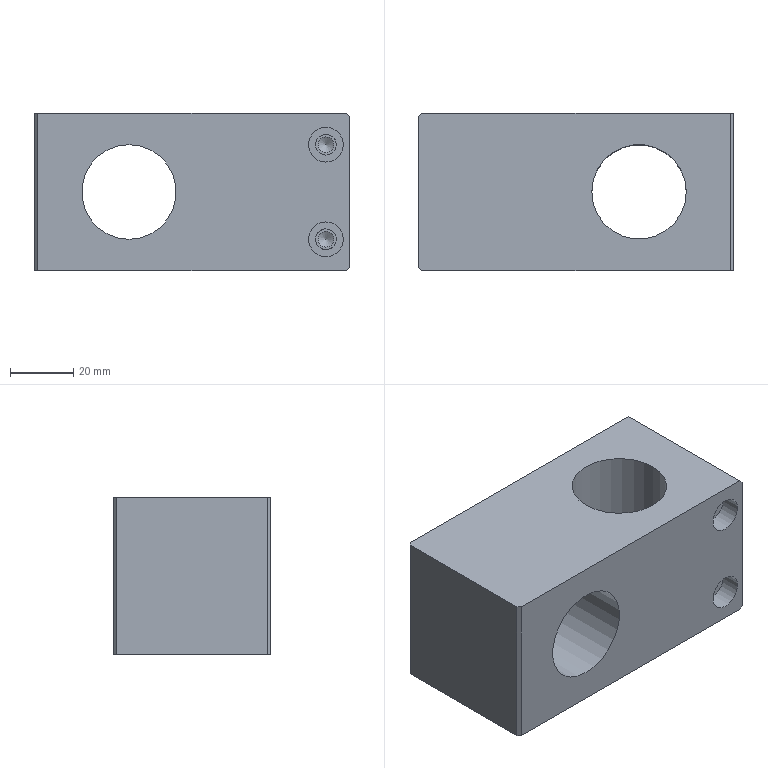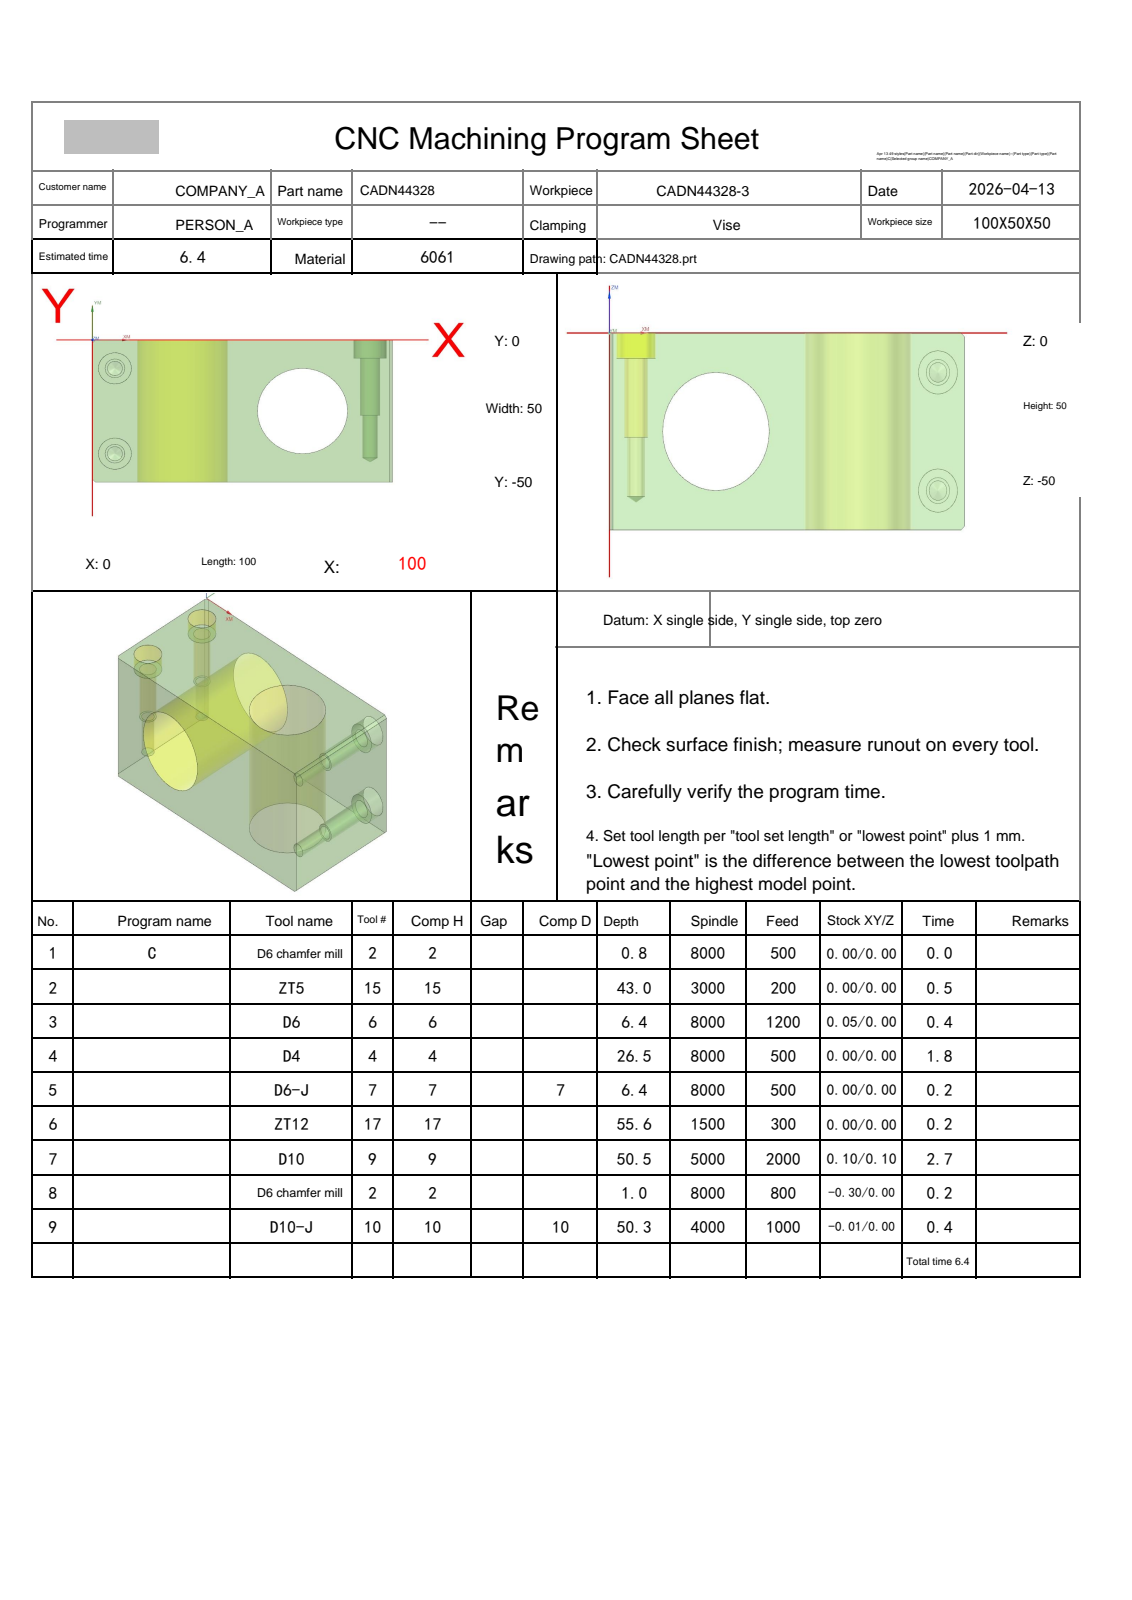NC program | NX | posted by the shop | part box 100 x 50 x 50 mm
Whole program:
%
O0001
(Machine time: 8.18 MIN)
(===Total Tool:8===)
(T2=D6 chamfer mill D=6. R=0. D- H02 Z=-1.   )
(T15=ZT5 D=5. DR_a=118 D- H15 Z=-43.  )
(T6=D6 D=6. R=0. D- H06 Z=-6.4  )
(T4=D4 D=4. R=0. D- H04 Z=-26.5 )
(T7=D6-J D=6. R=0. D7 H07 Z=-6.4  )
(T17=ZT12 D=12. DR_a=118 D- H17 Z=-55.61)
(T9=D10 D=10. R=0. D- H09 Z=-50.5 )
(T10=D10-J D=10. R=0. D10 H10 Z=-50.3 )
G80 G90 G17 G49 G40
G91 G28 Z0
M01
N1 T02 M06
(D6 chamfer mill D=6. R=0. H=02 ce=0.00 di=0.00)
G00 G90 G54 X7.5 Y-40. M03 S8000
G43 H02 Z20.
M08
G98 G81 X7.5 Y-40. Z-.8 R1. F500.
Y-10.
G80
G00 Z20.
G00 G90 X70. Y-25. M03 S8000
Z20.
G98 G82 X70. Y-25. Z-.8 R1. F500.
G80
G00 Z20.
G91 G28 Z0.0
M05
M09
G91 G28 Z0.0
M01
N2 T15 M06
(ZT5 D=5. DR_a=118 H=15)
G00 G90 G54 X7.5 Y-40. M03 S3000
G43 H15 Z20.
M08
G98 G83 X7.5 Y-40. Z-43.002 R1. F200. Q2.
Y-10.
G80
G00 Z20.
G91 G28 Z0.0
M05
M09
G91 G28 Z0.0
M01
N3 T06 M06
(D6 D=6. R=0. H=06 ce=0.05 di=0.00)
G00 G90 G54 X7.5 Y-40. M03 S8000
G43 H06 Z20.
M08
Z.5
G03 X8.725 Y-41.225 I1.225 J0.0 F1200.
X9.95 Y-40. I0.0 J1.225
X9.95 Y-40. Z0.0 I-2.45 J0.0
X9.95 Y-40. Z-.5 I-2.45 J0.0
X9.95 Y-40. Z-1. I-2.45 J0.0
X9.95 Y-40. Z-1.5 I-2.45 J0.0
X9.95 Y-40. Z-2. I-2.45 J0.0
X9.95 Y-40. Z-2.5 I-2.45 J0.0
X9.95 Y-40. Z-3. I-2.45 J0.0
X9.95 Y-40. Z-3.5 I-2.45 J0.0
X9.95 Y-40. Z-4. I-2.45 J0.0
X9.95 Y-40. Z-4.5 I-2.45 J0.0
X9.95 Y-40. Z-5. I-2.45 J0.0
X9.95 Y-40. Z-5.5 I-2.45 J0.0
X9.95 Y-40. Z-6. I-2.45 J0.0
X8.257 Y-42.33 Z-6.4 I-2.45 J0.0
X9.95 Y-40. I-.757 J2.33
X7.5 Y-37.55 I-2.45 J0.0
X5.05 Y-40. I0.0 J-2.45
X7.5 Y-42.45 I2.45 J0.0
X8.257 Y-42.33 I0.0 J2.45
X9.104 Y-41.165 I-.379 J1.165
X7.879 Y-39.94 I-1.225 J0.0
X7.5 Y-40. I0.0 J-1.225
G00 Z20.
Y-10.
Z.5
G03 X8.725 Y-11.225 I1.225 J0.0
X9.95 Y-10. I0.0 J1.225
X9.95 Y-10. Z0.0 I-2.45 J0.0
X9.95 Y-10. Z-.5 I-2.45 J0.0
X9.95 Y-10. Z-1. I-2.45 J0.0
X9.95 Y-10. Z-1.5 I-2.45 J0.0
X9.95 Y-10. Z-2. I-2.45 J0.0
X9.95 Y-10. Z-2.5 I-2.45 J0.0
X9.95 Y-10. Z-3. I-2.45 J0.0
X9.95 Y-10. Z-3.5 I-2.45 J0.0
X9.95 Y-10. Z-4. I-2.45 J0.0
X9.95 Y-10. Z-4.5 I-2.45 J0.0
X9.95 Y-10. Z-5. I-2.45 J0.0
X9.95 Y-10. Z-5.5 I-2.45 J0.0
X9.95 Y-10. Z-6. I-2.45 J0.0
X8.257 Y-12.33 Z-6.4 I-2.45 J0.0
X9.95 Y-10. I-.757 J2.33
X7.5 Y-7.55 I-2.45 J0.0
X5.05 Y-10. I0.0 J-2.45
X7.5 Y-12.45 I2.45 J0.0
X8.257 Y-12.33 I0.0 J2.45
X9.104 Y-11.165 I-.379 J1.165
X7.879 Y-9.94 I-1.225 J0.0
X7.5 Y-10. I0.0 J-1.225
G00 Z20.
G91 G28 Z0.0
M05
M09
G91 G28 Z0.0
M01
N4 T04 M06
(D4 D=4. R=0. H=04 ce=0.00 di=0.00)
G00 G90 G54 X7.5 Y-40. M03 S8000
G43 H04 Z20.
M08
Z-5.9
G03 X8.15 Y-40.65 I.65 J0.0 F500.
X8.8 Y-40. I0.0 J.65
X8.8 Y-40. Z-6.3 I-1.3 J0.0
X8.8 Y-40. Z-6.7 I-1.3 J0.0
X8.8 Y-40. Z-7.1 I-1.3 J0.0
X8.8 Y-40. Z-7.5 I-1.3 J0.0
X8.8 Y-40. Z-7.9 I-1.3 J0.0
X8.8 Y-40. Z-8.3 I-1.3 J0.0
X8.8 Y-40. Z-8.7 I-1.3 J0.0
X8.8 Y-40. Z-9.1 I-1.3 J0.0
X8.8 Y-40. Z-9.5 I-1.3 J0.0
X8.8 Y-40. Z-9.9 I-1.3 J0.0
X8.8 Y-40. Z-10.3 I-1.3 J0.0
X8.8 Y-40. Z-10.7 I-1.3 J0.0
X8.8 Y-40. Z-11.1 I-1.3 J0.0
X8.8 Y-40. Z-11.5 I-1.3 J0.0
X8.8 Y-40. Z-11.9 I-1.3 J0.0
X8.8 Y-40. Z-12.3 I-1.3 J0.0
X8.8 Y-40. Z-12.7 I-1.3 J0.0
X8.8 Y-40. Z-13.1 I-1.3 J0.0
X8.8 Y-40. Z-13.5 I-1.3 J0.0
X8.8 Y-40. Z-13.9 I-1.3 J0.0
X8.8 Y-40. Z-14.3 I-1.3 J0.0
X8.8 Y-40. Z-14.7 I-1.3 J0.0
X8.8 Y-40. Z-15.1 I-1.3 J0.0
X8.8 Y-40. Z-15.5 I-1.3 J0.0
X8.8 Y-40. Z-15.9 I-1.3 J0.0
X8.8 Y-40. Z-16.3 I-1.3 J0.0
X8.8 Y-40. Z-16.7 I-1.3 J0.0
X8.8 Y-40. Z-17.1 I-1.3 J0.0
X8.8 Y-40. Z-17.5 I-1.3 J0.0
X8.8 Y-40. Z-17.9 I-1.3 J0.0
X8.8 Y-40. Z-18.3 I-1.3 J0.0
X8.8 Y-40. Z-18.7 I-1.3 J0.0
X8.8 Y-40. Z-19.1 I-1.3 J0.0
X8.8 Y-40. Z-19.5 I-1.3 J0.0
X8.8 Y-40. Z-19.9 I-1.3 J0.0
X8.8 Y-40. Z-20.3 I-1.3 J0.0
X8.8 Y-40. Z-20.7 I-1.3 J0.0
X8.8 Y-40. Z-21.1 I-1.3 J0.0
X8.8 Y-40. Z-21.5 I-1.3 J0.0
X8.8 Y-40. Z-21.9 I-1.3 J0.0
X8.8 Y-40. Z-22.3 I-1.3 J0.0
X8.8 Y-40. Z-22.7 I-1.3 J0.0
X8.8 Y-40. Z-23.1 I-1.3 J0.0
X8.8 Y-40. Z-23.5 I-1.3 J0.0
X8.8 Y-40. Z-23.9 I-1.3 J0.0
X8.8 Y-40. Z-24.3 I-1.3 J0.0
X8.8 Y-40. Z-24.7 I-1.3 J0.0
X8.8 Y-40. Z-25.1 I-1.3 J0.0
X8.8 Y-40. Z-25.5 I-1.3 J0.0
X8.8 Y-40. Z-25.9 I-1.3 J0.0
X8.8 Y-40. Z-26.3 I-1.3 J0.0
X6.2 Y-40. Z-26.5 I-1.3 J0.0
X7.5 Y-41.3 I1.3 J0.0
X8.8 Y-40. I0.0 J1.3
X7.5 Y-38.7 I-1.3 J0.0
X6.2 Y-40. I0.0 J-1.3
X6.85 Y-40.65 I.65 J0.0
X7.5 Y-40. I0.0 J.65
G00 Z20.
Y-10.
Z-5.9
G03 X8.15 Y-10.65 I.65 J0.0
X8.8 Y-10. I0.0 J.65
X8.8 Y-10. Z-6.3 I-1.3 J0.0
X8.8 Y-10. Z-6.7 I-1.3 J0.0
X8.8 Y-10. Z-7.1 I-1.3 J0.0
X8.8 Y-10. Z-7.5 I-1.3 J0.0
X8.8 Y-10. Z-7.9 I-1.3 J0.0
X8.8 Y-10. Z-8.3 I-1.3 J0.0
X8.8 Y-10. Z-8.7 I-1.3 J0.0
X8.8 Y-10. Z-9.1 I-1.3 J0.0
X8.8 Y-10. Z-9.5 I-1.3 J0.0
X8.8 Y-10. Z-9.9 I-1.3 J0.0
X8.8 Y-10. Z-10.3 I-1.3 J0.0
X8.8 Y-10. Z-10.7 I-1.3 J0.0
X8.8 Y-10. Z-11.1 I-1.3 J0.0
X8.8 Y-10. Z-11.5 I-1.3 J0.0
X8.8 Y-10. Z-11.9 I-1.3 J0.0
X8.8 Y-10. Z-12.3 I-1.3 J0.0
X8.8 Y-10. Z-12.7 I-1.3 J0.0
X8.8 Y-10. Z-13.1 I-1.3 J0.0
X8.8 Y-10. Z-13.5 I-1.3 J0.0
X8.8 Y-10. Z-13.9 I-1.3 J0.0
X8.8 Y-10. Z-14.3 I-1.3 J0.0
X8.8 Y-10. Z-14.7 I-1.3 J0.0
X8.8 Y-10. Z-15.1 I-1.3 J0.0
X8.8 Y-10. Z-15.5 I-1.3 J0.0
X8.8 Y-10. Z-15.9 I-1.3 J0.0
X8.8 Y-10. Z-16.3 I-1.3 J0.0
X8.8 Y-10. Z-16.7 I-1.3 J0.0
X8.8 Y-10. Z-17.1 I-1.3 J0.0
X8.8 Y-10. Z-17.5 I-1.3 J0.0
X8.8 Y-10. Z-17.9 I-1.3 J0.0
X8.8 Y-10. Z-18.3 I-1.3 J0.0
X8.8 Y-10. Z-18.7 I-1.3 J0.0
X8.8 Y-10. Z-19.1 I-1.3 J0.0
X8.8 Y-10. Z-19.5 I-1.3 J0.0
X8.8 Y-10. Z-19.9 I-1.3 J0.0
X8.8 Y-10. Z-20.3 I-1.3 J0.0
X8.8 Y-10. Z-20.7 I-1.3 J0.0
X8.8 Y-10. Z-21.1 I-1.3 J0.0
X8.8 Y-10. Z-21.5 I-1.3 J0.0
X8.8 Y-10. Z-21.9 I-1.3 J0.0
X8.8 Y-10. Z-22.3 I-1.3 J0.0
X8.8 Y-10. Z-22.7 I-1.3 J0.0
X8.8 Y-10. Z-23.1 I-1.3 J0.0
X8.8 Y-10. Z-23.5 I-1.3 J0.0
X8.8 Y-10. Z-23.9 I-1.3 J0.0
X8.8 Y-10. Z-24.3 I-1.3 J0.0
X8.8 Y-10. Z-24.7 I-1.3 J0.0
X8.8 Y-10. Z-25.1 I-1.3 J0.0
X8.8 Y-10. Z-25.5 I-1.3 J0.0
X8.8 Y-10. Z-25.9 I-1.3 J0.0
X8.8 Y-10. Z-26.3 I-1.3 J0.0
X6.2 Y-10. Z-26.5 I-1.3 J0.0
X7.5 Y-11.3 I1.3 J0.0
X8.8 Y-10. I0.0 J1.3
X7.5 Y-8.7 I-1.3 J0.0
X6.2 Y-10. I0.0 J-1.3
X6.85 Y-10.65 I.65 J0.0
X7.5 Y-10. I0.0 J.65
G00 Z20.
G91 G28 Z0.0
M05
M09
G91 G28 Z0.0
M01
N5 T07 M06
(D6-J D=6. R=0. H=07 ce=0.00 di=0.00)
G00 G90 G54 X7.5 Y-40. M03 S8000
G43 H07 Z20.
M08
Z.5
G41 D07
G01 X7.532 Y-40.197 F500.
G03 X8.758 Y-41.242 I1.226 J.197
X10. Y-40. I0.0 J1.242
X10. Y-40. Z-4.5 I-2.5 J0.0
X5.678 Y-38.289 Z-6.4 I-2.5 J0.0
X5. Y-40. I1.822 J-1.711
X7.5 Y-42.5 I2.5 J0.0
X10. Y-40. I0.0 J2.5
X7.5 Y-37.5 I-2.5 J0.0
X5.678 Y-38.289 I0.0 J-2.5
X5.341 Y-39.139 I.905 J-.85
X6.583 Y-40.381 I1.242 J0.0
X7.342 Y-40.122 I0.0 J1.242
G01 G40 X7.5 Y-40.
G00 Z20.
Y-10.
Z.5
G41 D07
G01 X7.532 Y-10.197
G03 X8.758 Y-11.242 I1.226 J.197
X10. Y-10. I0.0 J1.242
X10. Y-10. Z-4.5 I-2.5 J0.0
X5.678 Y-8.289 Z-6.4 I-2.5 J0.0
X5. Y-10. I1.822 J-1.711
X7.5 Y-12.5 I2.5 J0.0
X10. Y-10. I0.0 J2.5
X7.5 Y-7.5 I-2.5 J0.0
X5.678 Y-8.289 I0.0 J-2.5
X5.341 Y-9.139 I.905 J-.85
X6.583 Y-10.381 I1.242 J0.0
X7.342 Y-10.122 I0.0 J1.242
G01 G40 X7.5 Y-10.
G00 Z20.
G91 G28 Z0.0
M05
M09
G91 G28 Z0.0
M01
N6 T17 M06
(ZT12 D=12. DR_a=118 H=17)
G00 G90 G54 X70. Y-25. M03 S1500
G43 H17 Z20.
M08
G98 G83 X70. Y-25. Z-55.605 R1. F300. Q3.
G80
G00 Z20.
G91 G28 Z0.0
M05
M09
G91 G28 Z0.0
M01
N7 T09 M06
(D10 D=10. R=0. H=09 ce=0.10 di=0.10)
G00 G90 G54 X60.729 Y-21.576 M03 S5000
G43 H09 Z20.
M08
Z1.
G01 X60.457 Y-22.256 Z.962 F2000.
X60.1 Y-24.229 Z.857
Y-25.771 Z.776
X60.457 Y-27.744 Z.671
X61.202 Y-29.604 Z.566
X62.306 Y-31.277 Z.461
X63.723 Y-32.694 Z.356
X65.396 Y-33.798 Z.251
X67.256 Y-34.543 Z.145
X69.229 Y-34.9 Z.04
X70. Z0.0
G03 X79.9 Y-25. Z-.149 I0.0 J9.9
X70. Y-15.1 Z-.297 I-9.9 J0.0
X60.1 Y-25. Z-.446 I0.0 J-9.9
X70. Y-34.9 Z-.594 I9.9 J0.0
X79.9 Y-25. Z-.743 I0.0 J9.9
X70. Y-15.1 Z-.891 I-9.9 J0.0
X60.1 Y-25. Z-1.04 I0.0 J-9.9
X70. Y-34.9 Z-1.188 I9.9 J0.0
X79.9 Y-25. Z-1.337 I0.0 J9.9
X70. Y-15.1 Z-1.485 I-9.9 J0.0
X60.1 Y-25. Z-1.634 I0.0 J-9.9
X70. Y-34.9 Z-1.782 I9.9 J0.0
X79.9 Y-25. Z-1.931 I0.0 J9.9
X70. Y-15.1 Z-2.079 I-9.9 J0.0
X60.1 Y-25. Z-2.228 I0.0 J-9.9
X70. Y-34.9 Z-2.376 I9.9 J0.0
X79.9 Y-25. Z-2.525 I0.0 J9.9
X70. Y-15.1 Z-2.674 I-9.9 J0.0
X60.1 Y-25. Z-2.822 I0.0 J-9.9
X70. Y-34.9 Z-2.971 I9.9 J0.0
X79.9 Y-25. Z-3.119 I0.0 J9.9
X70. Y-15.1 Z-3.268 I-9.9 J0.0
X60.1 Y-25. Z-3.416 I0.0 J-9.9
X70. Y-34.9 Z-3.565 I9.9 J0.0
X79.9 Y-25. Z-3.713 I0.0 J9.9
X70. Y-15.1 Z-3.862 I-9.9 J0.0
X60.1 Y-25. Z-4.01 I0.0 J-9.9
X70. Y-34.9 Z-4.159 I9.9 J0.0
X79.9 Y-25. Z-4.307 I0.0 J9.9
X70. Y-15.1 Z-4.456 I-9.9 J0.0
X60.1 Y-25. Z-4.604 I0.0 J-9.9
X70. Y-34.9 Z-4.753 I9.9 J0.0
X79.9 Y-25. Z-4.901 I0.0 J9.9
X70. Y-15.1 Z-5.05 I-9.9 J0.0
X60.1 Y-25. Z-5.199 I0.0 J-9.9
X70. Y-34.9 Z-5.347 I9.9 J0.0
X79.9 Y-25. Z-5.496 I0.0 J9.9
X70. Y-15.1 Z-5.644 I-9.9 J0.0
X60.1 Y-25. Z-5.793 I0.0 J-9.9
X70. Y-34.9 Z-5.941 I9.9 J0.0
X79.9 Y-25. Z-6.09 I0.0 J9.9
X70. Y-15.1 Z-6.238 I-9.9 J0.0
X60.1 Y-25. Z-6.387 I0.0 J-9.9
X70. Y-34.9 Z-6.535 I9.9 J0.0
X79.9 Y-25. Z-6.684 I0.0 J9.9
X70. Y-15.1 Z-6.832 I-9.9 J0.0
X60.1 Y-25. Z-6.981 I0.0 J-9.9
X70. Y-34.9 Z-7.129 I9.9 J0.0
X79.9 Y-25. Z-7.278 I0.0 J9.9
X70. Y-15.1 Z-7.426 I-9.9 J0.0
X60.1 Y-25. Z-7.575 I0.0 J-9.9
X70. Y-34.9 Z-7.724 I9.9 J0.0
X79.9 Y-25. Z-7.872 I0.0 J9.9
X70. Y-15.1 Z-8.021 I-9.9 J0.0
X60.1 Y-25. Z-8.169 I0.0 J-9.9
X70. Y-34.9 Z-8.318 I9.9 J0.0
X79.9 Y-25. Z-8.466 I0.0 J9.9
X70. Y-15.1 Z-8.615 I-9.9 J0.0
X60.1 Y-25. Z-8.763 I0.0 J-9.9
X70. Y-34.9 Z-8.912 I9.9 J0.0
X79.9 Y-25. Z-9.06 I0.0 J9.9
X70. Y-15.1 Z-9.209 I-9.9 J0.0
X60.1 Y-25. Z-9.357 I0.0 J-9.9
X70. Y-34.9 Z-9.506 I9.9 J0.0
X79.9 Y-25. Z-9.654 I0.0 J9.9
X70. Y-15.1 Z-9.803 I-9.9 J0.0
X60.1 Y-25. Z-9.951 I0.0 J-9.9
X70. Y-34.9 Z-10.1 I9.9 J0.0
X79.9 Y-25. Z-10.249 I0.0 J9.9
X70. Y-15.1 Z-10.397 I-9.9 J0.0
X60.1 Y-25. Z-10.546 I0.0 J-9.9
X70. Y-34.9 Z-10.694 I9.9 J0.0
X79.9 Y-25. Z-10.843 I0.0 J9.9
X70. Y-15.1 Z-10.991 I-9.9 J0.0
X60.1 Y-25. Z-11.14 I0.0 J-9.9
X70. Y-34.9 Z-11.288 I9.9 J0.0
X79.9 Y-25. Z-11.437 I0.0 J9.9
X70. Y-15.1 Z-11.585 I-9.9 J0.0
X60.1 Y-25. Z-11.734 I0.0 J-9.9
X70. Y-34.9 Z-11.882 I9.9 J0.0
X79.9 Y-25. Z-12.031 I0.0 J9.9
X70. Y-15.1 Z-12.179 I-9.9 J0.0
X60.1 Y-25. Z-12.328 I0.0 J-9.9
X70. Y-34.9 Z-12.476 I9.9 J0.0
X79.9 Y-25. Z-12.625 I0.0 J9.9
X70. Y-15.1 Z-12.774 I-9.9 J0.0
X60.1 Y-25. Z-12.922 I0.0 J-9.9
X70. Y-34.9 Z-13.071 I9.9 J0.0
X79.9 Y-25. Z-13.219 I0.0 J9.9
X70. Y-15.1 Z-13.368 I-9.9 J0.0
X60.1 Y-25. Z-13.516 I0.0 J-9.9
X70. Y-34.9 Z-13.665 I9.9 J0.0
X79.9 Y-25. Z-13.813 I0.0 J9.9
X70. Y-15.1 Z-13.962 I-9.9 J0.0
X60.1 Y-25. Z-14.11 I0.0 J-9.9
X70. Y-34.9 Z-14.259 I9.9 J0.0
X79.9 Y-25. Z-14.407 I0.0 J9.9
X70. Y-15.1 Z-14.556 I-9.9 J0.0
X60.1 Y-25. Z-14.704 I0.0 J-9.9
X70. Y-34.9 Z-14.853 I9.9 J0.0
X79.9 Y-25. Z-15.001 I0.0 J9.9
X70. Y-15.1 Z-15.15 I-9.9 J0.0
X60.1 Y-25. Z-15.299 I0.0 J-9.9
X70. Y-34.9 Z-15.447 I9.9 J0.0
X79.9 Y-25. Z-15.596 I0.0 J9.9
X70. Y-15.1 Z-15.744 I-9.9 J0.0
X60.1 Y-25. Z-15.893 I0.0 J-9.9
X70. Y-34.9 Z-16.041 I9.9 J0.0
X79.9 Y-25. Z-16.19 I0.0 J9.9
X70. Y-15.1 Z-16.338 I-9.9 J0.0
X60.1 Y-25. Z-16.487 I0.0 J-9.9
X70. Y-34.9 Z-16.635 I9.9 J0.0
X79.9 Y-25. Z-16.784 I0.0 J9.9
X70. Y-15.1 Z-16.932 I-9.9 J0.0
X60.1 Y-25. Z-17.081 I0.0 J-9.9
X70. Y-34.9 Z-17.229 I9.9 J0.0
X79.9 Y-25. Z-17.378 I0.0 J9.9
X70. Y-15.1 Z-17.526 I-9.9 J0.0
X60.1 Y-25. Z-17.675 I0.0 J-9.9
X70. Y-34.9 Z-17.824 I9.9 J0.0
X79.9 Y-25. Z-17.972 I0.0 J9.9
X70. Y-15.1 Z-18.121 I-9.9 J0.0
X60.1 Y-25. Z-18.269 I0.0 J-9.9
X70. Y-34.9 Z-18.418 I9.9 J0.0
X79.9 Y-25. Z-18.566 I0.0 J9.9
X70. Y-15.1 Z-18.715 I-9.9 J0.0
X60.1 Y-25. Z-18.863 I0.0 J-9.9
X70. Y-34.9 Z-19.012 I9.9 J0.0
X79.9 Y-25. Z-19.16 I0.0 J9.9
X70. Y-15.1 Z-19.309 I-9.9 J0.0
X60.1 Y-25. Z-19.457 I0.0 J-9.9
X70. Y-34.9 Z-19.606 I9.9 J0.0
X79.9 Y-25. Z-19.754 I0.0 J9.9
X70. Y-15.1 Z-19.903 I-9.9 J0.0
X60.1 Y-25. Z-20.051 I0.0 J-9.9
X70. Y-34.9 Z-20.2 I9.9 J0.0
X79.9 Y-25. Z-20.349 I0.0 J9.9
X70. Y-15.1 Z-20.497 I-9.9 J0.0
X60.1 Y-25. Z-20.646 I0.0 J-9.9
X70. Y-34.9 Z-20.794 I9.9 J0.0
X79.9 Y-25. Z-20.943 I0.0 J9.9
X70. Y-15.1 Z-21.091 I-9.9 J0.0
X60.1 Y-25. Z-21.24 I0.0 J-9.9
X70. Y-34.9 Z-21.388 I9.9 J0.0
X79.9 Y-25. Z-21.537 I0.0 J9.9
X70. Y-15.1 Z-21.685 I-9.9 J0.0
X60.1 Y-25. Z-21.834 I0.0 J-9.9
X70. Y-34.9 Z-21.982 I9.9 J0.0
X79.9 Y-25. Z-22.131 I0.0 J9.9
X70. Y-15.1 Z-22.279 I-9.9 J0.0
X60.1 Y-25. Z-22.428 I0.0 J-9.9
X70. Y-34.9 Z-22.576 I9.9 J0.0
X79.9 Y-25. Z-22.725 I0.0 J9.9
X70. Y-15.1 Z-22.874 I-9.9 J0.0
X60.1 Y-25. Z-23.022 I0.0 J-9.9
X70. Y-34.9 Z-23.171 I9.9 J0.0
X79.9 Y-25. Z-23.319 I0.0 J9.9
X70. Y-15.1 Z-23.468 I-9.9 J0.0
X60.1 Y-25. Z-23.616 I0.0 J-9.9
X70. Y-34.9 Z-23.765 I9.9 J0.0
X79.9 Y-25. Z-23.913 I0.0 J9.9
X70. Y-15.1 Z-24.062 I-9.9 J0.0
X60.1 Y-25. Z-24.21 I0.0 J-9.9
X70. Y-34.9 Z-24.359 I9.9 J0.0
X79.9 Y-25. Z-24.507 I0.0 J9.9
X70. Y-15.1 Z-24.656 I-9.9 J0.0
X60.1 Y-25. Z-24.804 I0.0 J-9.9
X70. Y-34.9 Z-24.953 I9.9 J0.0
X79.9 Y-25. Z-25.101 I0.0 J9.9
X70. Y-15.1 Z-25.25 I-9.9 J0.0
X60.1 Y-25. Z-25.399 I0.0 J-9.9
X70. Y-34.9 Z-25.547 I9.9 J0.0
X79.9 Y-25. Z-25.696 I0.0 J9.9
X70. Y-15.1 Z-25.844 I-9.9 J0.0
X60.1 Y-25. Z-25.993 I0.0 J-9.9
X70. Y-34.9 Z-26.141 I9.9 J0.0
X79.9 Y-25. Z-26.29 I0.0 J9.9
X70. Y-15.1 Z-26.438 I-9.9 J0.0
X60.1 Y-25. Z-26.587 I0.0 J-9.9
X70. Y-34.9 Z-26.735 I9.9 J0.0
X79.9 Y-25. Z-26.884 I0.0 J9.9
X70. Y-15.1 Z-27.032 I-9.9 J0.0
X60.1 Y-25. Z-27.181 I0.0 J-9.9
X70. Y-34.9 Z-27.329 I9.9 J0.0
X79.9 Y-25. Z-27.478 I0.0 J9.9
X70. Y-15.1 Z-27.626 I-9.9 J0.0
X60.1 Y-25. Z-27.775 I0.0 J-9.9
X70. Y-34.9 Z-27.924 I9.9 J0.0
X79.9 Y-25. Z-28.072 I0.0 J9.9
X70. Y-15.1 Z-28.221 I-9.9 J0.0
X60.1 Y-25. Z-28.369 I0.0 J-9.9
X70. Y-34.9 Z-28.518 I9.9 J0.0
X79.9 Y-25. Z-28.666 I0.0 J9.9
X70. Y-15.1 Z-28.815 I-9.9 J0.0
X60.1 Y-25. Z-28.963 I0.0 J-9.9
X70. Y-34.9 Z-29.112 I9.9 J0.0
X79.9 Y-25. Z-29.26 I0.0 J9.9
X70. Y-15.1 Z-29.409 I-9.9 J0.0
X60.1 Y-25. Z-29.557 I0.0 J-9.9
X70. Y-34.9 Z-29.706 I9.9 J0.0
X79.9 Y-25. Z-29.854 I0.0 J9.9
X70. Y-15.1 Z-30.003 I-9.9 J0.0
X60.1 Y-25. Z-30.151 I0.0 J-9.9
X70. Y-34.9 Z-30.3 I9.9 J0.0
X79.9 Y-25. Z-30.449 I0.0 J9.9
X70. Y-15.1 Z-30.597 I-9.9 J0.0
X60.1 Y-25. Z-30.746 I0.0 J-9.9
X70. Y-34.9 Z-30.894 I9.9 J0.0
X79.9 Y-25. Z-31.043 I0.0 J9.9
X70. Y-15.1 Z-31.191 I-9.9 J0.0
X60.1 Y-25. Z-31.34 I0.0 J-9.9
X70. Y-34.9 Z-31.488 I9.9 J0.0
X79.9 Y-25. Z-31.637 I0.0 J9.9
X70. Y-15.1 Z-31.785 I-9.9 J0.0
X60.1 Y-25. Z-31.934 I0.0 J-9.9
X70. Y-34.9 Z-32.082 I9.9 J0.0
X79.9 Y-25. Z-32.231 I0.0 J9.9
X70. Y-15.1 Z-32.379 I-9.9 J0.0
X60.1 Y-25. Z-32.528 I0.0 J-9.9
X70. Y-34.9 Z-32.676 I9.9 J0.0
X79.9 Y-25. Z-32.825 I0.0 J9.9
X70. Y-15.1 Z-32.974 I-9.9 J0.0
X60.1 Y-25. Z-33.122 I0.0 J-9.9
X70. Y-34.9 Z-33.271 I9.9 J0.0
X79.9 Y-25. Z-33.419 I0.0 J9.9
X70. Y-15.1 Z-33.568 I-9.9 J0.0
X60.1 Y-25. Z-33.716 I0.0 J-9.9
X70. Y-34.9 Z-33.865 I9.9 J0.0
X79.9 Y-25. Z-34.013 I0.0 J9.9
X70. Y-15.1 Z-34.162 I-9.9 J0.0
X60.1 Y-25. Z-34.31 I0.0 J-9.9
X70. Y-34.9 Z-34.459 I9.9 J0.0
X79.9 Y-25. Z-34.607 I0.0 J9.9
X70. Y-15.1 Z-34.756 I-9.9 J0.0
X60.1 Y-25. Z-34.904 I0.0 J-9.9
X70. Y-34.9 Z-35.053 I9.9 J0.0
X79.9 Y-25. Z-35.201 I0.0 J9.9
X70. Y-15.1 Z-35.35 I-9.9 J0.0
X60.1 Y-25. Z-35.499 I0.0 J-9.9
X70. Y-34.9 Z-35.647 I9.9 J0.0
X79.9 Y-25. Z-35.796 I0.0 J9.9
X70. Y-15.1 Z-35.944 I-9.9 J0.0
X60.1 Y-25. Z-36.093 I0.0 J-9.9
X70. Y-34.9 Z-36.241 I9.9 J0.0
X79.9 Y-25. Z-36.39 I0.0 J9.9
X70. Y-15.1 Z-36.538 I-9.9 J0.0
X60.1 Y-25. Z-36.687 I0.0 J-9.9
X70. Y-34.9 Z-36.835 I9.9 J0.0
X79.9 Y-25. Z-36.984 I0.0 J9.9
X70. Y-15.1 Z-37.132 I-9.9 J0.0
X60.1 Y-25. Z-37.281 I0.0 J-9.9
X70. Y-34.9 Z-37.429 I9.9 J0.0
X79.9 Y-25. Z-37.578 I0.0 J9.9
X70. Y-15.1 Z-37.726 I-9.9 J0.0
X60.1 Y-25. Z-37.875 I0.0 J-9.9
X70. Y-34.9 Z-38.024 I9.9 J0.0
X79.9 Y-25. Z-38.172 I0.0 J9.9
X70. Y-15.1 Z-38.321 I-9.9 J0.0
X60.1 Y-25. Z-38.469 I0.0 J-9.9
X70. Y-34.9 Z-38.618 I9.9 J0.0
X79.9 Y-25. Z-38.766 I0.0 J9.9
X70. Y-15.1 Z-38.915 I-9.9 J0.0
X60.1 Y-25. Z-39.063 I0.0 J-9.9
X70. Y-34.9 Z-39.212 I9.9 J0.0
X79.9 Y-25. Z-39.36 I0.0 J9.9
X70. Y-15.1 Z-39.509 I-9.9 J0.0
X60.1 Y-25. Z-39.657 I0.0 J-9.9
X70. Y-34.9 Z-39.806 I9.9 J0.0
X79.9 Y-25. Z-39.954 I0.0 J9.9
X70. Y-15.1 Z-40.103 I-9.9 J0.0
X60.1 Y-25. Z-40.251 I0.0 J-9.9
X70. Y-34.9 Z-40.4 I9.9 J0.0
X79.9 Y-25. Z-40.549 I0.0 J9.9
X70. Y-15.1 Z-40.697 I-9.9 J0.0
X60.1 Y-25. Z-40.846 I0.0 J-9.9
X70. Y-34.9 Z-40.994 I9.9 J0.0
X79.9 Y-25. Z-41.143 I0.0 J9.9
X70. Y-15.1 Z-41.291 I-9.9 J0.0
X60.1 Y-25. Z-41.44 I0.0 J-9.9
X70. Y-34.9 Z-41.588 I9.9 J0.0
X79.9 Y-25. Z-41.737 I0.0 J9.9
X70. Y-15.1 Z-41.885 I-9.9 J0.0
X60.1 Y-25. Z-42.034 I0.0 J-9.9
X70. Y-34.9 Z-42.182 I9.9 J0.0
X79.9 Y-25. Z-42.331 I0.0 J9.9
X70. Y-15.1 Z-42.479 I-9.9 J0.0
X60.1 Y-25. Z-42.628 I0.0 J-9.9
X70. Y-34.9 Z-42.776 I9.9 J0.0
X79.9 Y-25. Z-42.925 I0.0 J9.9
X70. Y-15.1 Z-43.074 I-9.9 J0.0
X60.1 Y-25. Z-43.222 I0.0 J-9.9
X70. Y-34.9 Z-43.371 I9.9 J0.0
X79.9 Y-25. Z-43.519 I0.0 J9.9
X70. Y-15.1 Z-43.668 I-9.9 J0.0
X60.1 Y-25. Z-43.816 I0.0 J-9.9
X70. Y-34.9 Z-43.965 I9.9 J0.0
X79.9 Y-25. Z-44.113 I0.0 J9.9
X70. Y-15.1 Z-44.262 I-9.9 J0.0
X60.1 Y-25. Z-44.41 I0.0 J-9.9
X70. Y-34.9 Z-44.559 I9.9 J0.0
X79.9 Y-25. Z-44.707 I0.0 J9.9
X70. Y-15.1 Z-44.856 I-9.9 J0.0
X60.1 Y-25. Z-45.004 I0.0 J-9.9
X70. Y-34.9 Z-45.153 I9.9 J0.0
X79.9 Y-25. Z-45.301 I0.0 J9.9
X70. Y-15.1 Z-45.45 I-9.9 J0.0
X60.1 Y-25. Z-45.599 I0.0 J-9.9
X70. Y-34.9 Z-45.747 I9.9 J0.0
X79.9 Y-25. Z-45.896 I0.0 J9.9
X70. Y-15.1 Z-46.044 I-9.9 J0.0
X60.1 Y-25. Z-46.193 I0.0 J-9.9
X70. Y-34.9 Z-46.341 I9.9 J0.0
X79.9 Y-25. Z-46.49 I0.0 J9.9
X70. Y-15.1 Z-46.638 I-9.9 J0.0
X60.1 Y-25. Z-46.787 I0.0 J-9.9
X70. Y-34.9 Z-46.935 I9.9 J0.0
X79.9 Y-25. Z-47.084 I0.0 J9.9
X70. Y-15.1 Z-47.232 I-9.9 J0.0
X60.1 Y-25. Z-47.381 I0.0 J-9.9
X70. Y-34.9 Z-47.529 I9.9 J0.0
X79.9 Y-25. Z-47.678 I0.0 J9.9
X70. Y-15.1 Z-47.826 I-9.9 J0.0
X60.1 Y-25. Z-47.975 I0.0 J-9.9
X70. Y-34.9 Z-48.124 I9.9 J0.0
X79.9 Y-25. Z-48.272 I0.0 J9.9
X70. Y-15.1 Z-48.421 I-9.9 J0.0
X60.1 Y-25. Z-48.569 I0.0 J-9.9
X70. Y-34.9 Z-48.718 I9.9 J0.0
X79.9 Y-25. Z-48.866 I0.0 J9.9
X70. Y-15.1 Z-49.015 I-9.9 J0.0
X60.1 Y-25. Z-49.163 I0.0 J-9.9
X70. Y-34.9 Z-49.312 I9.9 J0.0
X79.9 Y-25. Z-49.46 I0.0 J9.9
X70. Y-15.1 Z-49.609 I-9.9 J0.0
X60.1 Y-25. Z-49.757 I0.0 J-9.9
X70. Y-34.9 Z-49.906 I9.9 J0.0
X79.9 Y-25. Z-50.054 I0.0 J9.9
X70. Y-15.1 Z-50.203 I-9.9 J0.0
X60.1 Y-25. Z-50.351 I0.0 J-9.9
X70. Y-34.9 Z-50.5 I9.9 J0.0
X79.9 Y-25. I0.0 J9.9
X70. Y-15.1 I-9.9 J0.0
X60.1 Y-25. I0.0 J-9.9
X70. Y-34.9 I9.9 J0.0
X70.4 Y-34.892 I0.0 J9.9
G01 Z-49.5
G00 Z20.
G91 G28 Z0.0
M05
M09
G91 G28 Z0.0
M01
N8 T02 M06
(D6 chamfer mill D=6. R=0. H=02 ce=-0.30 di=0.00)
G00 G90 G54 X9.3 Y-43. M03 S8000
G43 H02 Z20.
M08
Z-.5
G01 Z-1. F800.
G03 X12.3 Y-40. I0.0 J3.
X7.5 Y-35.2 I-4.8 J0.0
X2.7 Y-40. I0.0 J-4.8
X7.5 Y-44.8 I4.8 J0.0
X12.3 Y-40. I0.0 J4.8
X9.3 Y-37. I-3. J0.0
G01 Z-.5
G00 Z20.
Y-13.
Z-.5
G01 Z-1.
G03 X12.3 Y-10. I0.0 J3.
X7.5 Y-5.2 I-4.8 J0.0
X2.7 Y-10. I0.0 J-4.8
X7.5 Y-14.8 I4.8 J0.0
X12.3 Y-10. I0.0 J4.8
X9.3 Y-7. I-3. J0.0
G01 Z-.5
G00 Z20.
G00 G90 X58.7 Y-22. M03 S8000
Z20.
Z-.5
G01 Z-1. F800.
G03 X55.7 Y-25. I0.0 J-3.
X70. Y-39.3 I14.3 J0.0
X84.3 Y-25. I0.0 J14.3
X70. Y-10.7 I-14.3 J0.0
X55.7 Y-25. I0.0 J-14.3
X58.7 Y-28. I3. J0.0
G01 Z-.5
G00 Z20.
G91 G28 Z0.0
M05
M09
G91 G28 Z0.0
M01
N9 T10 M06
(D10-J D=10. R=0. H=10 ce=-0.01 di=0.00)
G00 G90 G54 X68.5 Y-33.177 M03 S4000
G43 H10 Z10.
M08
Z-6.883
G01 Z-8.383 F1000.
G41 D10
Y-33.51
G03 X70. Y-35.01 I1.5 J0.0
X80.01 Y-25. I0.0 J10.01
X70. Y-14.99 I-10.01 J0.0
X59.99 Y-25. I0.0 J-10.01
X70. Y-35.01 I10.01 J0.0
X70.4 Y-35.002 I0.0 J10.01
X71.84 Y-33.503 I-.06 J1.499
G01 X71.839 Y-33.443
X71.833 Y-33.31
G40 X71.825 Y-33.11
Z-6.883
G00 X68.5 Y-33.177
Z-15.267
G01 Z-16.767
G41 D10
Y-33.51
G03 X70. Y-35.01 I1.5 J0.0
X80.01 Y-25. I0.0 J10.01
X70. Y-14.99 I-10.01 J0.0
X59.99 Y-25. I0.0 J-10.01
X70. Y-35.01 I10.01 J0.0
X70.4 Y-35.002 I0.0 J10.01
X71.84 Y-33.503 I-.06 J1.499
G01 X71.839 Y-33.443
X71.833 Y-33.31
G40 X71.825 Y-33.11
Z-15.267
G00 X68.5 Y-33.177
Z-23.65
G01 Z-25.15
G41 D10
Y-33.51
G03 X70. Y-35.01 I1.5 J0.0
X80.01 Y-25. I0.0 J10.01
X70. Y-14.99 I-10.01 J0.0
X59.99 Y-25. I0.0 J-10.01
X70. Y-35.01 I10.01 J0.0
X70.4 Y-35.002 I0.0 J10.01
X71.84 Y-33.503 I-.06 J1.499
G01 X71.839 Y-33.443
X71.833 Y-33.31
G40 X71.825 Y-33.11
Z-23.65
G00 X68.5 Y-33.177
Z-32.033
G01 Z-33.533
G41 D10
Y-33.51
G03 X70. Y-35.01 I1.5 J0.0
X80.01 Y-25. I0.0 J10.01
X70. Y-14.99 I-10.01 J0.0
X59.99 Y-25. I0.0 J-10.01
X70. Y-35.01 I10.01 J0.0
X70.4 Y-35.002 I0.0 J10.01
X71.84 Y-33.503 I-.06 J1.499
G01 X71.839 Y-33.443
X71.833 Y-33.31
G40 X71.825 Y-33.11
Z-32.033
G00 X68.5 Y-33.177
Z-40.417
G01 Z-41.917
G41 D10
Y-33.51
G03 X70. Y-35.01 I1.5 J0.0
X80.01 Y-25. I0.0 J10.01
X70. Y-14.99 I-10.01 J0.0
X59.99 Y-25. I0.0 J-10.01
X70. Y-35.01 I10.01 J0.0
X70.4 Y-35.002 I0.0 J10.01
X71.84 Y-33.503 I-.06 J1.499
G01 X71.839 Y-33.443
X71.833 Y-33.31
G40 X71.825 Y-33.11
Z-40.417
G00 X68.5 Y-33.177
Z-48.8
G01 Z-50.3
G41 D10
Y-33.51
G03 X70. Y-35.01 I1.5 J0.0
X80.01 Y-25. I0.0 J10.01
X70. Y-14.99 I-10.01 J0.0
X59.99 Y-25. I0.0 J-10.01
X70. Y-35.01 I10.01 J0.0
X70.4 Y-35.002 I0.0 J10.01
X71.84 Y-33.503 I-.06 J1.499
G01 X71.839 Y-33.443
X71.833 Y-33.31
G40 X71.825 Y-33.11
Z-48.8
G00 Z10.
M05
M09
G91 G28 Z0.0
G91 G28 Y0.0
M30
%